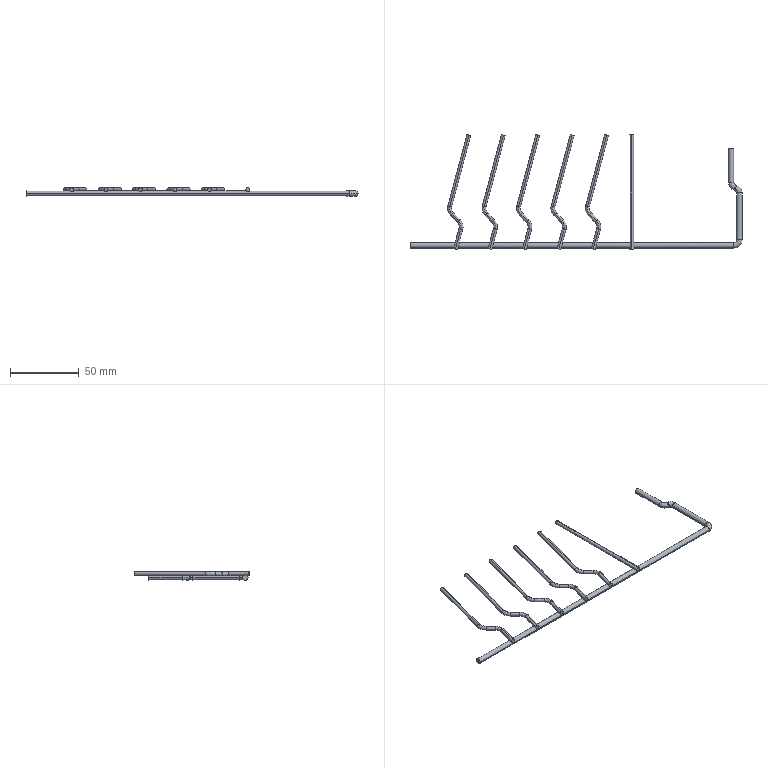Part | STEP file | ZXW735-L-178-A_11_1_1 | 1 solid | 80 faces | box 240.95 x 83.325 x 6.203 mm | volume 6917 mm3 | cylinder 40 | torus 26 | plane 14 | commonest cylinder face diameters 2.8 x32 3.9 x8